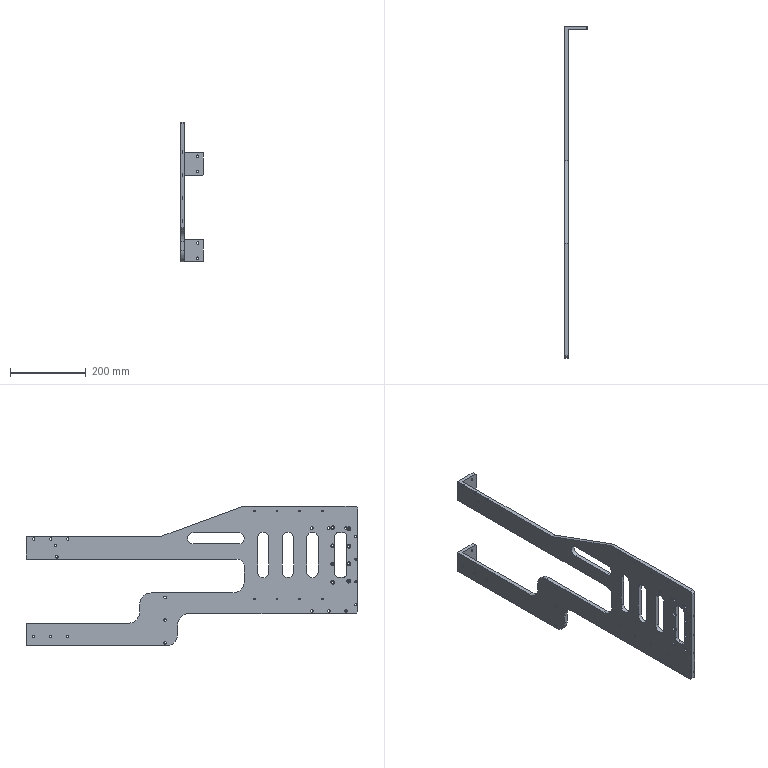Part | STEP file | longitudinal seal film pull fixing plate_SUS304 | 1 solid | 232 faces | box 60 x 876 x 369 mm | volume 1562891 mm3 | cylinder 165 | plane 67 | commonest cylinder face diameters 6.6 x35 11 x35 5.5 x25 10 x25 4.2 x16 30 x11